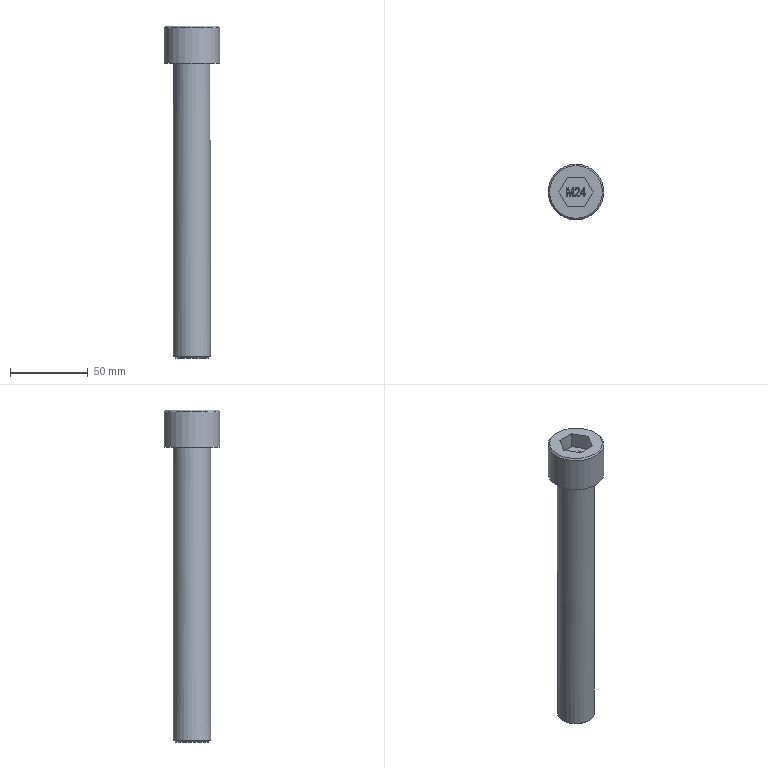Part | STEP file | M24-1 | 1 solid | 51 faces | box 36 x 36 x 214 mm | volume 107145 mm3 | plane 43 | other 4 | cylinder 2 | cone 2 | commonest cylinder face diameters 24 x1 36 x1